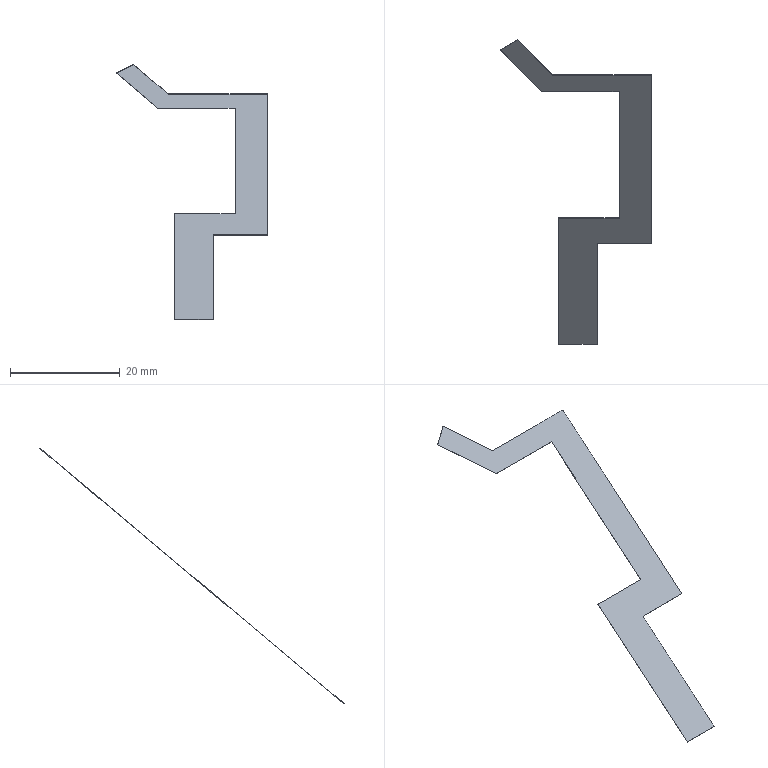Part | SolidWorks | features BaseBody 1 | 1 solid | 15 faces | box 27.714 x 55.483 x 46.567 mm | volume 28.639 mm3 | plane 15
STEP:
#1=CARTESIAN_POINT('',(-699.451,644.234,358.166));
#2=VERTEX_POINT('',#1);
#3=CARTESIAN_POINT('',(-699.451,644.267,358.127));
#4=VERTEX_POINT('',#3);
#5=CARTESIAN_POINT('',(-699.451,644.234,358.166));
#6=DIRECTION('',(-0.000000993,0.6428,-0.766));
#7=VECTOR('',#6,1000.);
#8=LINE('',#5,#7);
#9=EDGE_CURVE('',#2,#4,#8,.T.);
#10=ORIENTED_EDGE('',*,*,#9,.F.);
#11=CARTESIAN_POINT('',(-699.451,667.216,377.449));
#12=VERTEX_POINT('',#11);
#13=CARTESIAN_POINT('',(-699.451,667.216,377.449));
#14=DIRECTION('',(0.000001286,-0.766,-0.6428));
#15=VECTOR('',#14,1000.);
#16=LINE('',#13,#15);
#17=EDGE_CURVE('',#12,#2,#16,.T.);
#18=ORIENTED_EDGE('',*,*,#17,.F.);
#19=CARTESIAN_POINT('',(-699.451,667.248,377.411));
#20=VERTEX_POINT('',#19);
#21=CARTESIAN_POINT('',(-699.451,667.248,377.411));
#22=DIRECTION('',(0.000000993,-0.6428,0.766));
#23=VECTOR('',#22,1000.);
#24=LINE('',#21,#23);
#25=EDGE_CURVE('',#20,#12,#24,.T.);
#26=ORIENTED_EDGE('',*,*,#25,.F.);
#27=CARTESIAN_POINT('',(-699.451,644.267,358.127));
#28=DIRECTION('',(-0.000001286,0.766,0.6428));
#29=VECTOR('',#28,1000.);
#30=LINE('',#27,#29);
#31=EDGE_CURVE('',#4,#20,#30,.T.);
#32=ORIENTED_EDGE('',*,*,#31,.F.);
#33=EDGE_LOOP('',(#10,#18,#26,#32));
#34=FACE_OUTER_BOUND('',#33,.T.);
#35=CARTESIAN_POINT('',(-699.451,648.863,361.984));
#36=DIRECTION('',(1.,0.000001623,0.000000066));
#37=DIRECTION('',(0.000000993,-0.6428,0.766));
#38=AXIS2_PLACEMENT_3D('',#35,#36,#37);
#39=PLANE('',#38);
#40=ADVANCED_FACE('',(#34),#39,.F.);
#41=CARTESIAN_POINT('',(-688.451,690.229,396.695));
#42=VERTEX_POINT('',#41);
#43=CARTESIAN_POINT('',(-702.645,690.229,396.695));
#44=VERTEX_POINT('',#43);
#45=CARTESIAN_POINT('',(-688.451,690.229,396.695));
#46=DIRECTION('',(-1.,-0.000001822,-0.000000233));
#47=VECTOR('',#46,1000.);
#48=LINE('',#45,#47);
#49=EDGE_CURVE('',#42,#44,#48,.T.);
#50=ORIENTED_EDGE('',*,*,#49,.T.);
#51=CARTESIAN_POINT('',(-710.165,697.873,403.109));
#52=VERTEX_POINT('',#51);
#53=CARTESIAN_POINT('',(-710.165,697.873,403.109));
#54=DIRECTION('',(0.6018,-0.6118,-0.5134));
#55=VECTOR('',#54,1000.);
#56=LINE('',#53,#55);
#57=EDGE_CURVE('',#52,#44,#56,.T.);
#58=ORIENTED_EDGE('',*,*,#57,.F.);
#59=CARTESIAN_POINT('',(-706.97,699.717,404.656));
#60=VERTEX_POINT('',#59);
#61=CARTESIAN_POINT('',(-706.97,699.717,404.656));
#62=DIRECTION('',(-0.7986,-0.461,-0.3868));
#63=VECTOR('',#62,1000.);
#64=LINE('',#61,#63);
#65=EDGE_CURVE('',#60,#52,#64,.T.);
#66=ORIENTED_EDGE('',*,*,#65,.F.);
#67=CARTESIAN_POINT('',(-700.651,693.293,399.266));
#68=VERTEX_POINT('',#67);
#69=CARTESIAN_POINT('',(-700.651,693.293,399.266));
#70=DIRECTION('',(-0.6018,0.6118,0.5134));
#71=VECTOR('',#70,1000.);
#72=LINE('',#69,#71);
#73=EDGE_CURVE('',#68,#60,#72,.T.);
#74=ORIENTED_EDGE('',*,*,#73,.F.);
#75=CARTESIAN_POINT('',(-688.451,693.293,399.266));
#76=VERTEX_POINT('',#75);
#77=CARTESIAN_POINT('',(-688.451,693.293,399.266));
#78=DIRECTION('',(-1.,-0.000001865,-0.000000268));
#79=VECTOR('',#78,1000.);
#80=LINE('',#77,#79);
#81=EDGE_CURVE('',#76,#68,#80,.T.);
#82=ORIENTED_EDGE('',*,*,#81,.F.);
#83=CARTESIAN_POINT('',(-682.451,693.294,399.266));
#84=VERTEX_POINT('',#83);
#85=CARTESIAN_POINT('',(-682.451,693.294,399.266));
#86=DIRECTION('',(-1.,-0.000001661,-0.000000097));
#87=VECTOR('',#86,1000.);
#88=LINE('',#85,#87);
#89=EDGE_CURVE('',#84,#76,#88,.T.);
#90=ORIENTED_EDGE('',*,*,#89,.F.);
#91=CARTESIAN_POINT('',(-682.451,662.652,373.554));
#92=VERTEX_POINT('',#91);
#93=CARTESIAN_POINT('',(-682.451,662.652,373.554));
#94=DIRECTION('',(-0.000001286,0.766,0.6428));
#95=VECTOR('',#94,1000.);
#96=LINE('',#93,#95);
#97=EDGE_CURVE('',#92,#84,#96,.T.);
#98=ORIENTED_EDGE('',*,*,#97,.F.);
#99=CARTESIAN_POINT('',(-692.451,662.652,373.554));
#100=VERTEX_POINT('',#99);
#101=CARTESIAN_POINT('',(-692.451,662.652,373.554));
#102=DIRECTION('',(1.,0.000001623,0.000000066));
#103=VECTOR('',#102,1000.);
#104=LINE('',#101,#103);
#105=EDGE_CURVE('',#100,#92,#104,.T.);
#106=ORIENTED_EDGE('',*,*,#105,.F.);
#107=CARTESIAN_POINT('',(-692.451,644.267,358.127));
#108=VERTEX_POINT('',#107);
#109=CARTESIAN_POINT('',(-692.451,644.267,358.127));
#110=DIRECTION('',(-0.000001286,0.766,0.6428));
#111=VECTOR('',#110,1000.);
#112=LINE('',#109,#111);
#113=EDGE_CURVE('',#108,#100,#112,.T.);
#114=ORIENTED_EDGE('',*,*,#113,.F.);
#115=CARTESIAN_POINT('',(-699.451,644.267,358.127));
#116=DIRECTION('',(1.,0.000001623,0.000000066));
#117=VECTOR('',#116,1000.);
#118=LINE('',#115,#117);
#119=EDGE_CURVE('',#4,#108,#118,.T.);
#120=ORIENTED_EDGE('',*,*,#119,.F.);
#121=ORIENTED_EDGE('',*,*,#31,.T.);
#122=CARTESIAN_POINT('',(-688.451,667.248,377.411));
#123=VERTEX_POINT('',#122);
#124=CARTESIAN_POINT('',(-699.451,667.248,377.411));
#125=DIRECTION('',(1.,0.000001623,0.000000066));
#126=VECTOR('',#125,1000.);
#127=LINE('',#124,#126);
#128=EDGE_CURVE('',#20,#123,#127,.T.);
#129=ORIENTED_EDGE('',*,*,#128,.T.);
#130=CARTESIAN_POINT('',(-688.451,667.248,377.411));
#131=DIRECTION('',(-0.000001286,0.766,0.6428));
#132=VECTOR('',#131,1000.);
#133=LINE('',#130,#132);
#134=EDGE_CURVE('',#123,#42,#133,.T.);
#135=ORIENTED_EDGE('',*,*,#134,.T.);
#136=EDGE_LOOP('',(#50,#58,#66,#74,#82,#90,#98,#106,#114,#120,#121,#129,#135));
#137=FACE_OUTER_BOUND('',#136,.T.);
#138=CARTESIAN_POINT('',(-733.13,689.217,395.846));
#139=DIRECTION('',(-0.000000993,0.6428,-0.766));
#140=DIRECTION('',(1.,0.000001623,0.000000066));
#141=AXIS2_PLACEMENT_3D('',#138,#139,#140);
#142=PLANE('',#141);
#143=ADVANCED_FACE('',(#137),#142,.T.);
#144=CARTESIAN_POINT('',(-688.451,667.216,377.449));
#145=VERTEX_POINT('',#144);
#146=CARTESIAN_POINT('',(-688.451,667.248,377.411));
#147=DIRECTION('',(0.000000993,-0.6428,0.766));
#148=VECTOR('',#147,1000.);
#149=LINE('',#146,#148);
#150=EDGE_CURVE('',#123,#145,#149,.T.);
#151=ORIENTED_EDGE('',*,*,#150,.T.);
#152=CARTESIAN_POINT('',(-688.451,690.197,396.733));
#153=VERTEX_POINT('',#152);
#154=CARTESIAN_POINT('',(-688.451,667.216,377.449));
#155=DIRECTION('',(-0.000001286,0.766,0.6428));
#156=VECTOR('',#155,1000.);
#157=LINE('',#154,#156);
#158=EDGE_CURVE('',#145,#153,#157,.T.);
#159=ORIENTED_EDGE('',*,*,#158,.T.);
#160=CARTESIAN_POINT('',(-688.451,690.229,396.695));
#161=DIRECTION('',(0.000000993,-0.6428,0.766));
#162=VECTOR('',#161,1000.);
#163=LINE('',#160,#162);
#164=EDGE_CURVE('',#42,#153,#163,.T.);
#165=ORIENTED_EDGE('',*,*,#164,.F.);
#166=ORIENTED_EDGE('',*,*,#134,.F.);
#167=EDGE_LOOP('',(#151,#159,#165,#166));
#168=FACE_OUTER_BOUND('',#167,.T.);
#169=CARTESIAN_POINT('',(-688.451,693.293,399.266));
#170=DIRECTION('',(-1.,-0.000001623,-0.000000066));
#171=DIRECTION('',(0.000000993,-0.6428,0.766));
#172=AXIS2_PLACEMENT_3D('',#169,#170,#171);
#173=PLANE('',#172);
#174=ADVANCED_FACE('',(#168),#173,.T.);
#175=ORIENTED_EDGE('',*,*,#49,.F.);
#176=ORIENTED_EDGE('',*,*,#164,.T.);
#177=CARTESIAN_POINT('',(-702.645,690.197,396.733));
#178=VERTEX_POINT('',#177);
#179=CARTESIAN_POINT('',(-688.451,690.197,396.733));
#180=DIRECTION('',(-1.,-0.000001822,-0.000000233));
#181=VECTOR('',#180,1000.);
#182=LINE('',#179,#181);
#183=EDGE_CURVE('',#153,#178,#182,.T.);
#184=ORIENTED_EDGE('',*,*,#183,.T.);
#185=CARTESIAN_POINT('',(-702.645,690.229,396.695));
#186=DIRECTION('',(0.000000993,-0.6428,0.766));
#187=VECTOR('',#186,1000.);
#188=LINE('',#185,#187);
#189=EDGE_CURVE('',#44,#178,#188,.T.);
#190=ORIENTED_EDGE('',*,*,#189,.F.);
#191=EDGE_LOOP('',(#175,#176,#184,#190));
#192=FACE_OUTER_BOUND('',#191,.T.);
#193=CARTESIAN_POINT('',(-688.451,690.229,396.695));
#194=DIRECTION('',(-0.000001866,0.766,0.6428));
#195=DIRECTION('',(-1.,-0.000002068,-0.000000439));
#196=AXIS2_PLACEMENT_3D('',#193,#194,#195);
#197=PLANE('',#196);
#198=ADVANCED_FACE('',(#192),#197,.F.);
#199=ORIENTED_EDGE('',*,*,#57,.T.);
#200=ORIENTED_EDGE('',*,*,#189,.T.);
#201=CARTESIAN_POINT('',(-710.165,697.841,403.147));
#202=VERTEX_POINT('',#201);
#203=CARTESIAN_POINT('',(-702.645,690.197,396.733));
#204=DIRECTION('',(-0.6018,0.6118,0.5134));
#205=VECTOR('',#204,1000.);
#206=LINE('',#203,#205);
#207=EDGE_CURVE('',#178,#202,#206,.T.);
#208=ORIENTED_EDGE('',*,*,#207,.T.);
#209=CARTESIAN_POINT('',(-710.165,697.841,403.147));
#210=DIRECTION('',(-0.000000993,0.6428,-0.766));
#211=VECTOR('',#210,1000.);
#212=LINE('',#209,#211);
#213=EDGE_CURVE('',#202,#52,#212,.T.);
#214=ORIENTED_EDGE('',*,*,#213,.T.);
#215=EDGE_LOOP('',(#199,#200,#208,#214));
#216=FACE_OUTER_BOUND('',#215,.T.);
#217=CARTESIAN_POINT('',(-702.645,690.229,396.695));
#218=DIRECTION('',(0.7986,0.461,0.3868));
#219=DIRECTION('',(-0.6018,0.6118,0.5134));
#220=AXIS2_PLACEMENT_3D('',#217,#218,#219);
#221=PLANE('',#220);
#222=ADVANCED_FACE('',(#216),#221,.F.);
#223=ORIENTED_EDGE('',*,*,#65,.T.);
#224=ORIENTED_EDGE('',*,*,#213,.F.);
#225=CARTESIAN_POINT('',(-706.97,699.685,404.694));
#226=VERTEX_POINT('',#225);
#227=CARTESIAN_POINT('',(-710.165,697.841,403.147));
#228=DIRECTION('',(0.7986,0.461,0.3868));
#229=VECTOR('',#228,1000.);
#230=LINE('',#227,#229);
#231=EDGE_CURVE('',#202,#226,#230,.T.);
#232=ORIENTED_EDGE('',*,*,#231,.T.);
#233=CARTESIAN_POINT('',(-706.97,699.685,404.694));
#234=DIRECTION('',(-0.000000993,0.6428,-0.766));
#235=VECTOR('',#234,1000.);
#236=LINE('',#233,#235);
#237=EDGE_CURVE('',#226,#60,#236,.T.);
#238=ORIENTED_EDGE('',*,*,#237,.T.);
#239=EDGE_LOOP('',(#223,#224,#232,#238));
#240=FACE_OUTER_BOUND('',#239,.T.);
#241=CARTESIAN_POINT('',(-710.165,697.873,403.109));
#242=DIRECTION('',(0.6018,-0.6118,-0.5134));
#243=DIRECTION('',(0.7986,0.461,0.3868));
#244=AXIS2_PLACEMENT_3D('',#241,#242,#243);
#245=PLANE('',#244);
#246=ADVANCED_FACE('',(#240),#245,.F.);
#247=ORIENTED_EDGE('',*,*,#73,.T.);
#248=ORIENTED_EDGE('',*,*,#237,.F.);
#249=CARTESIAN_POINT('',(-700.651,693.261,399.304));
#250=VERTEX_POINT('',#249);
#251=CARTESIAN_POINT('',(-706.97,699.685,404.694));
#252=DIRECTION('',(0.6018,-0.6118,-0.5134));
#253=VECTOR('',#252,1000.);
#254=LINE('',#251,#253);
#255=EDGE_CURVE('',#226,#250,#254,.T.);
#256=ORIENTED_EDGE('',*,*,#255,.T.);
#257=CARTESIAN_POINT('',(-700.651,693.261,399.304));
#258=DIRECTION('',(-0.000000993,0.6428,-0.766));
#259=VECTOR('',#258,1000.);
#260=LINE('',#257,#259);
#261=EDGE_CURVE('',#250,#68,#260,.T.);
#262=ORIENTED_EDGE('',*,*,#261,.T.);
#263=EDGE_LOOP('',(#247,#248,#256,#262));
#264=FACE_OUTER_BOUND('',#263,.T.);
#265=CARTESIAN_POINT('',(-706.97,699.717,404.656));
#266=DIRECTION('',(-0.7986,-0.461,-0.3868));
#267=DIRECTION('',(0.6018,-0.6118,-0.5134));
#268=AXIS2_PLACEMENT_3D('',#265,#266,#267);
#269=PLANE('',#268);
#270=ADVANCED_FACE('',(#264),#269,.F.);
#271=ORIENTED_EDGE('',*,*,#81,.T.);
#272=ORIENTED_EDGE('',*,*,#261,.F.);
#273=CARTESIAN_POINT('',(-688.451,693.261,399.304));
#274=VERTEX_POINT('',#273);
#275=CARTESIAN_POINT('',(-700.651,693.261,399.304));
#276=DIRECTION('',(1.,0.000001865,0.000000268));
#277=VECTOR('',#276,1000.);
#278=LINE('',#275,#277);
#279=EDGE_CURVE('',#250,#274,#278,.T.);
#280=ORIENTED_EDGE('',*,*,#279,.T.);
#281=CARTESIAN_POINT('',(-688.451,693.261,399.304));
#282=DIRECTION('',(-0.000000993,0.6428,-0.766));
#283=VECTOR('',#282,1000.);
#284=LINE('',#281,#283);
#285=EDGE_CURVE('',#274,#76,#284,.T.);
#286=ORIENTED_EDGE('',*,*,#285,.T.);
#287=EDGE_LOOP('',(#271,#272,#280,#286));
#288=FACE_OUTER_BOUND('',#287,.T.);
#289=CARTESIAN_POINT('',(-700.651,693.293,399.266));
#290=DIRECTION('',(0.000001866,-0.766,-0.6428));
#291=DIRECTION('',(1.,0.000002068,0.000000439));
#292=AXIS2_PLACEMENT_3D('',#289,#290,#291);
#293=PLANE('',#292);
#294=ADVANCED_FACE('',(#288),#293,.F.);
#295=ORIENTED_EDGE('',*,*,#89,.T.);
#296=ORIENTED_EDGE('',*,*,#285,.F.);
#297=CARTESIAN_POINT('',(-682.451,693.261,399.304));
#298=VERTEX_POINT('',#297);
#299=CARTESIAN_POINT('',(-688.451,693.261,399.304));
#300=DIRECTION('',(1.,0.000001661,0.000000097));
#301=VECTOR('',#300,1000.);
#302=LINE('',#299,#301);
#303=EDGE_CURVE('',#274,#298,#302,.T.);
#304=ORIENTED_EDGE('',*,*,#303,.T.);
#305=CARTESIAN_POINT('',(-682.451,693.261,399.304));
#306=DIRECTION('',(-0.000000993,0.6428,-0.766));
#307=VECTOR('',#306,1000.);
#308=LINE('',#305,#307);
#309=EDGE_CURVE('',#298,#84,#308,.T.);
#310=ORIENTED_EDGE('',*,*,#309,.T.);
#311=EDGE_LOOP('',(#295,#296,#304,#310));
#312=FACE_OUTER_BOUND('',#311,.T.);
#313=CARTESIAN_POINT('',(-680.451,693.294,399.266));
#314=DIRECTION('',(-0.000001286,0.766,0.6428));
#315=DIRECTION('',(-0.000000993,0.6428,-0.766));
#316=AXIS2_PLACEMENT_3D('',#313,#314,#315);
#317=PLANE('',#316);
#318=ADVANCED_FACE('',(#312),#317,.T.);
#319=ORIENTED_EDGE('',*,*,#97,.T.);
#320=ORIENTED_EDGE('',*,*,#309,.F.);
#321=CARTESIAN_POINT('',(-682.451,662.62,373.593));
#322=VERTEX_POINT('',#321);
#323=CARTESIAN_POINT('',(-682.451,693.261,399.304));
#324=DIRECTION('',(0.000001286,-0.766,-0.6428));
#325=VECTOR('',#324,1000.);
#326=LINE('',#323,#325);
#327=EDGE_CURVE('',#298,#322,#326,.T.);
#328=ORIENTED_EDGE('',*,*,#327,.T.);
#329=CARTESIAN_POINT('',(-682.451,662.62,373.593));
#330=DIRECTION('',(-0.000000993,0.6428,-0.766));
#331=VECTOR('',#330,1000.);
#332=LINE('',#329,#331);
#333=EDGE_CURVE('',#322,#92,#332,.T.);
#334=ORIENTED_EDGE('',*,*,#333,.T.);
#335=EDGE_LOOP('',(#319,#320,#328,#334));
#336=FACE_OUTER_BOUND('',#335,.T.);
#337=CARTESIAN_POINT('',(-682.451,667.248,377.411));
#338=DIRECTION('',(1.,0.000001623,0.000000066));
#339=DIRECTION('',(-0.000000993,0.6428,-0.766));
#340=AXIS2_PLACEMENT_3D('',#337,#338,#339);
#341=PLANE('',#340);
#342=ADVANCED_FACE('',(#336),#341,.T.);
#343=ORIENTED_EDGE('',*,*,#333,.F.);
#344=CARTESIAN_POINT('',(-692.451,662.62,373.593));
#345=VERTEX_POINT('',#344);
#346=CARTESIAN_POINT('',(-682.451,662.62,373.593));
#347=DIRECTION('',(-1.,-0.000001623,-0.000000066));
#348=VECTOR('',#347,1000.);
#349=LINE('',#346,#348);
#350=EDGE_CURVE('',#322,#345,#349,.T.);
#351=ORIENTED_EDGE('',*,*,#350,.T.);
#352=CARTESIAN_POINT('',(-692.451,662.62,373.593));
#353=DIRECTION('',(-0.000000993,0.6428,-0.766));
#354=VECTOR('',#353,1000.);
#355=LINE('',#352,#354);
#356=EDGE_CURVE('',#345,#100,#355,.T.);
#357=ORIENTED_EDGE('',*,*,#356,.T.);
#358=ORIENTED_EDGE('',*,*,#105,.T.);
#359=EDGE_LOOP('',(#343,#351,#357,#358));
#360=FACE_OUTER_BOUND('',#359,.T.);
#361=CARTESIAN_POINT('',(-697.451,662.652,373.554));
#362=DIRECTION('',(0.000001286,-0.766,-0.6428));
#363=DIRECTION('',(0.000000993,-0.6428,0.766));
#364=AXIS2_PLACEMENT_3D('',#361,#362,#363);
#365=PLANE('',#364);
#366=ADVANCED_FACE('',(#360),#365,.T.);
#367=CARTESIAN_POINT('',(-692.451,644.235,358.166));
#368=VERTEX_POINT('',#367);
#369=CARTESIAN_POINT('',(-692.451,662.62,373.593));
#370=DIRECTION('',(0.000001286,-0.766,-0.6428));
#371=VECTOR('',#370,1000.);
#372=LINE('',#369,#371);
#373=EDGE_CURVE('',#345,#368,#372,.T.);
#374=ORIENTED_EDGE('',*,*,#373,.T.);
#375=CARTESIAN_POINT('',(-692.451,644.235,358.166));
#376=DIRECTION('',(-0.000000993,0.6428,-0.766));
#377=VECTOR('',#376,1000.);
#378=LINE('',#375,#377);
#379=EDGE_CURVE('',#368,#108,#378,.T.);
#380=ORIENTED_EDGE('',*,*,#379,.T.);
#381=ORIENTED_EDGE('',*,*,#113,.T.);
#382=ORIENTED_EDGE('',*,*,#356,.F.);
#383=EDGE_LOOP('',(#374,#380,#381,#382));
#384=FACE_OUTER_BOUND('',#383,.T.);
#385=CARTESIAN_POINT('',(-692.451,671.844,381.268));
#386=DIRECTION('',(-1.,-0.000001623,-0.000000066));
#387=DIRECTION('',(-0.000000993,0.6428,-0.766));
#388=AXIS2_PLACEMENT_3D('',#385,#386,#387);
#389=PLANE('',#388);
#390=ADVANCED_FACE('',(#384),#389,.F.);
#391=ORIENTED_EDGE('',*,*,#119,.T.);
#392=ORIENTED_EDGE('',*,*,#379,.F.);
#393=CARTESIAN_POINT('',(-692.451,644.235,358.166));
#394=DIRECTION('',(-1.,-0.000001623,-0.000000066));
#395=VECTOR('',#394,1000.);
#396=LINE('',#393,#395);
#397=EDGE_CURVE('',#368,#2,#396,.T.);
#398=ORIENTED_EDGE('',*,*,#397,.T.);
#399=ORIENTED_EDGE('',*,*,#9,.T.);
#400=EDGE_LOOP('',(#391,#392,#398,#399));
#401=FACE_OUTER_BOUND('',#400,.T.);
#402=CARTESIAN_POINT('',(-690.451,644.267,358.127));
#403=DIRECTION('',(-0.000001286,0.766,0.6428));
#404=DIRECTION('',(0.000000993,-0.6428,0.766));
#405=AXIS2_PLACEMENT_3D('',#402,#403,#404);
#406=PLANE('',#405);
#407=ADVANCED_FACE('',(#401),#406,.F.);
#408=ORIENTED_EDGE('',*,*,#397,.F.);
#409=ORIENTED_EDGE('',*,*,#373,.F.);
#410=ORIENTED_EDGE('',*,*,#350,.F.);
#411=ORIENTED_EDGE('',*,*,#327,.F.);
#412=ORIENTED_EDGE('',*,*,#303,.F.);
#413=ORIENTED_EDGE('',*,*,#279,.F.);
#414=ORIENTED_EDGE('',*,*,#255,.F.);
#415=ORIENTED_EDGE('',*,*,#231,.F.);
#416=ORIENTED_EDGE('',*,*,#207,.F.);
#417=ORIENTED_EDGE('',*,*,#183,.F.);
#418=ORIENTED_EDGE('',*,*,#158,.F.);
#419=CARTESIAN_POINT('',(-688.451,667.216,377.449));
#420=DIRECTION('',(-1.,-0.000001623,-0.000000066));
#421=VECTOR('',#420,1000.);
#422=LINE('',#419,#421);
#423=EDGE_CURVE('',#145,#12,#422,.T.);
#424=ORIENTED_EDGE('',*,*,#423,.T.);
#425=ORIENTED_EDGE('',*,*,#17,.T.);
#426=EDGE_LOOP('',(#408,#409,#410,#411,#412,#413,#414,#415,#416,#417,#418,#424,#425));
#427=FACE_OUTER_BOUND('',#426,.T.);
#428=CARTESIAN_POINT('',(-733.13,684.589,392.027));
#429=DIRECTION('',(-0.000000993,0.6428,-0.766));
#430=DIRECTION('',(1.,0.000001623,0.000000066));
#431=AXIS2_PLACEMENT_3D('',#428,#429,#430);
#432=PLANE('',#431);
#433=ADVANCED_FACE('',(#427),#432,.F.);
#434=ORIENTED_EDGE('',*,*,#128,.F.);
#435=ORIENTED_EDGE('',*,*,#25,.T.);
#436=ORIENTED_EDGE('',*,*,#423,.F.);
#437=ORIENTED_EDGE('',*,*,#150,.F.);
#438=EDGE_LOOP('',(#434,#435,#436,#437));
#439=FACE_OUTER_BOUND('',#438,.T.);
#440=CARTESIAN_POINT('',(-697.451,667.248,377.411));
#441=DIRECTION('',(0.000001286,-0.766,-0.6428));
#442=DIRECTION('',(-0.000000993,0.6428,-0.766));
#443=AXIS2_PLACEMENT_3D('',#440,#441,#442);
#444=PLANE('',#443);
#445=ADVANCED_FACE('',(#439),#444,.F.);
#446=CLOSED_SHELL('',(#40,#143,#174,#198,#222,#246,#270,#294,#318,#342,#366,#390,#407,#433,#445));
#447=MANIFOLD_SOLID_BREP('',#446);
#448=CARTESIAN_POINT('',(0.,0.,0.));
#449=DIRECTION('',(0.,0.,1.));
#450=DIRECTION('',(1.,0.,0.));
#451=AXIS2_PLACEMENT_3D('',#448,#449,#450);
#452=(LENGTH_UNIT()NAMED_UNIT(*)SI_UNIT(.MILLI.,.METRE.));
#453=UNCERTAINTY_MEASURE_WITH_UNIT(LENGTH_MEASURE(0.00001),#452,'','');
#454=(NAMED_UNIT(*)PLANE_ANGLE_UNIT()SI_UNIT($,.RADIAN.));
#455=(NAMED_UNIT(*)SI_UNIT($,.STERADIAN.)SOLID_ANGLE_UNIT());
#456=(GEOMETRIC_REPRESENTATION_CONTEXT(3)GLOBAL_UNCERTAINTY_ASSIGNED_CONTEXT((#453))GLOBAL_UNIT_ASSIGNED_CONTEXT((#452,#454,#455))REPRESENTATION_CONTEXT('',''));
#457=ADVANCED_BREP_SHAPE_REPRESENTATION('',(#447,#451),#456);